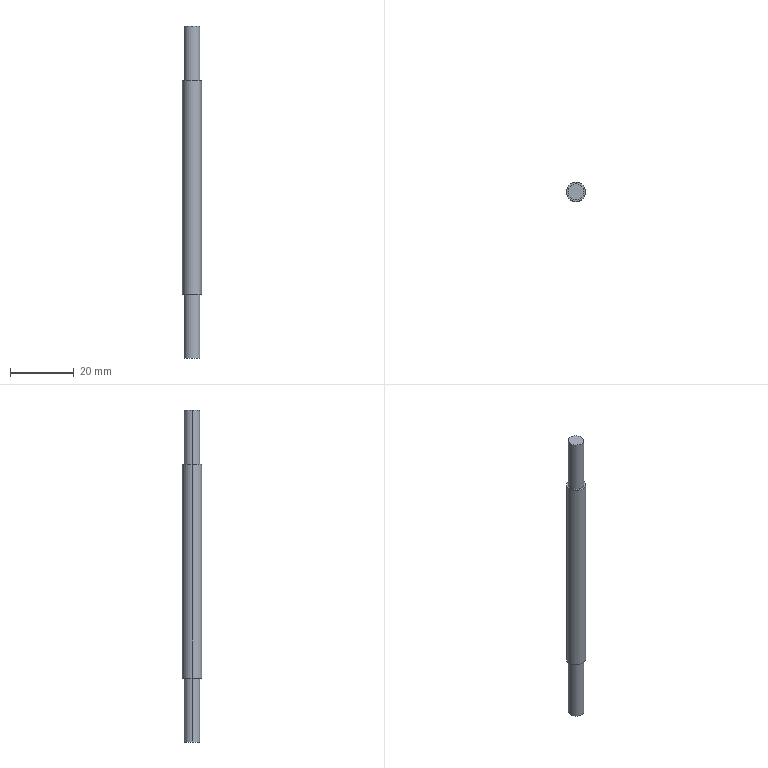Part | SolidWorks | features ICE 2, Extrusion 1 | 1 solid | 10 faces | box 6 x 6 x 104 mm | volume 2621 mm3 | cylinder 6 | plane 4 | commonest cylinder face diameters 5 x4 6 x2
STEP:
#1=CARTESIAN_POINT('',(2.5,0.,104.));
#2=VERTEX_POINT('',#1);
#3=CARTESIAN_POINT('',(-2.5,0.,104.));
#4=VERTEX_POINT('',#3);
#5=CARTESIAN_POINT('',(0.,0.,104.));
#6=DIRECTION('',(0.,0.,1.));
#7=DIRECTION('',(1.,0.,0.));
#8=AXIS2_PLACEMENT_3D('',#5,#6,#7);
#9=CIRCLE('',#8,2.5);
#10=EDGE_CURVE('',#2,#4,#9,.T.);
#11=ORIENTED_EDGE('',*,*,#10,.F.);
#12=CARTESIAN_POINT('',(2.5,0.,87.));
#13=VERTEX_POINT('',#12);
#14=CARTESIAN_POINT('',(2.5,0.,104.));
#15=DIRECTION('',(0.,0.,-1.));
#16=VECTOR('',#15,1000.);
#17=LINE('',#14,#16);
#18=EDGE_CURVE('',#2,#13,#17,.T.);
#19=ORIENTED_EDGE('',*,*,#18,.T.);
#20=CARTESIAN_POINT('',(-2.5,0.,87.));
#21=VERTEX_POINT('',#20);
#22=CARTESIAN_POINT('',(0.,0.,87.));
#23=DIRECTION('',(0.,0.,1.));
#24=DIRECTION('',(1.,0.,0.));
#25=AXIS2_PLACEMENT_3D('',#22,#23,#24);
#26=CIRCLE('',#25,2.5);
#27=EDGE_CURVE('',#13,#21,#26,.T.);
#28=ORIENTED_EDGE('',*,*,#27,.T.);
#29=CARTESIAN_POINT('',(-2.5,0.,104.));
#30=DIRECTION('',(0.,0.,-1.));
#31=VECTOR('',#30,1000.);
#32=LINE('',#29,#31);
#33=EDGE_CURVE('',#4,#21,#32,.T.);
#34=ORIENTED_EDGE('',*,*,#33,.F.);
#35=EDGE_LOOP('',(#11,#19,#28,#34));
#36=FACE_OUTER_BOUND('',#35,.T.);
#37=CARTESIAN_POINT('',(0.,0.,104.));
#38=DIRECTION('',(0.,0.,-1.));
#39=DIRECTION('',(-1.,0.,0.));
#40=AXIS2_PLACEMENT_3D('',#37,#38,#39);
#41=CYLINDRICAL_SURFACE('',#40,2.5);
#42=ADVANCED_FACE('',(#36),#41,.T.);
#43=CARTESIAN_POINT('',(3.,0.,87.));
#44=VERTEX_POINT('',#43);
#45=CARTESIAN_POINT('',(-3.,0.,87.));
#46=VERTEX_POINT('',#45);
#47=CARTESIAN_POINT('',(0.,0.,87.));
#48=DIRECTION('',(0.,0.,1.));
#49=DIRECTION('',(1.,0.,0.));
#50=AXIS2_PLACEMENT_3D('',#47,#48,#49);
#51=CIRCLE('',#50,3.);
#52=EDGE_CURVE('',#44,#46,#51,.T.);
#53=ORIENTED_EDGE('',*,*,#52,.F.);
#54=CARTESIAN_POINT('',(3.,0.,20.));
#55=VERTEX_POINT('',#54);
#56=CARTESIAN_POINT('',(3.,0.,87.));
#57=DIRECTION('',(0.,0.,-1.));
#58=VECTOR('',#57,1000.);
#59=LINE('',#56,#58);
#60=EDGE_CURVE('',#44,#55,#59,.T.);
#61=ORIENTED_EDGE('',*,*,#60,.T.);
#62=CARTESIAN_POINT('',(-3.,0.,20.));
#63=VERTEX_POINT('',#62);
#64=CARTESIAN_POINT('',(0.,0.,20.));
#65=DIRECTION('',(0.,0.,1.));
#66=DIRECTION('',(1.,0.,0.));
#67=AXIS2_PLACEMENT_3D('',#64,#65,#66);
#68=CIRCLE('',#67,3.);
#69=EDGE_CURVE('',#55,#63,#68,.T.);
#70=ORIENTED_EDGE('',*,*,#69,.T.);
#71=CARTESIAN_POINT('',(-3.,0.,87.));
#72=DIRECTION('',(0.,0.,-1.));
#73=VECTOR('',#72,1000.);
#74=LINE('',#71,#73);
#75=EDGE_CURVE('',#46,#63,#74,.T.);
#76=ORIENTED_EDGE('',*,*,#75,.F.);
#77=EDGE_LOOP('',(#53,#61,#70,#76));
#78=FACE_OUTER_BOUND('',#77,.T.);
#79=CARTESIAN_POINT('',(0.,0.,87.));
#80=DIRECTION('',(0.,0.,-1.));
#81=DIRECTION('',(-1.,0.,0.));
#82=AXIS2_PLACEMENT_3D('',#79,#80,#81);
#83=CYLINDRICAL_SURFACE('',#82,3.);
#84=ADVANCED_FACE('',(#78),#83,.T.);
#85=CARTESIAN_POINT('',(2.5,0.,20.));
#86=VERTEX_POINT('',#85);
#87=CARTESIAN_POINT('',(-2.5,0.,20.));
#88=VERTEX_POINT('',#87);
#89=CARTESIAN_POINT('',(0.,0.,20.));
#90=DIRECTION('',(0.,0.,1.));
#91=DIRECTION('',(1.,0.,0.));
#92=AXIS2_PLACEMENT_3D('',#89,#90,#91);
#93=CIRCLE('',#92,2.5);
#94=EDGE_CURVE('',#86,#88,#93,.T.);
#95=ORIENTED_EDGE('',*,*,#94,.F.);
#96=CARTESIAN_POINT('',(2.5,0.,0.));
#97=VERTEX_POINT('',#96);
#98=CARTESIAN_POINT('',(2.5,0.,20.));
#99=DIRECTION('',(0.,0.,-1.));
#100=VECTOR('',#99,1000.);
#101=LINE('',#98,#100);
#102=EDGE_CURVE('',#86,#97,#101,.T.);
#103=ORIENTED_EDGE('',*,*,#102,.T.);
#104=CARTESIAN_POINT('',(-2.5,0.,0.));
#105=VERTEX_POINT('',#104);
#106=CARTESIAN_POINT('',(0.,0.,0.));
#107=DIRECTION('',(0.,0.,1.));
#108=DIRECTION('',(1.,0.,0.));
#109=AXIS2_PLACEMENT_3D('',#106,#107,#108);
#110=CIRCLE('',#109,2.5);
#111=EDGE_CURVE('',#97,#105,#110,.T.);
#112=ORIENTED_EDGE('',*,*,#111,.T.);
#113=CARTESIAN_POINT('',(-2.5,0.,20.));
#114=DIRECTION('',(0.,0.,-1.));
#115=VECTOR('',#114,1000.);
#116=LINE('',#113,#115);
#117=EDGE_CURVE('',#88,#105,#116,.T.);
#118=ORIENTED_EDGE('',*,*,#117,.F.);
#119=EDGE_LOOP('',(#95,#103,#112,#118));
#120=FACE_OUTER_BOUND('',#119,.T.);
#121=CARTESIAN_POINT('',(0.,0.,20.));
#122=DIRECTION('',(0.,0.,-1.));
#123=DIRECTION('',(-1.,0.,0.));
#124=AXIS2_PLACEMENT_3D('',#121,#122,#123);
#125=CYLINDRICAL_SURFACE('',#124,2.5);
#126=ADVANCED_FACE('',(#120),#125,.T.);
#127=ORIENTED_EDGE('',*,*,#102,.F.);
#128=CARTESIAN_POINT('',(0.,0.,20.));
#129=DIRECTION('',(0.,0.,1.));
#130=DIRECTION('',(1.,0.,0.));
#131=AXIS2_PLACEMENT_3D('',#128,#129,#130);
#132=CIRCLE('',#131,2.5);
#133=EDGE_CURVE('',#88,#86,#132,.T.);
#134=ORIENTED_EDGE('',*,*,#133,.F.);
#135=ORIENTED_EDGE('',*,*,#117,.T.);
#136=CARTESIAN_POINT('',(0.,0.,0.));
#137=DIRECTION('',(0.,0.,1.));
#138=DIRECTION('',(1.,0.,0.));
#139=AXIS2_PLACEMENT_3D('',#136,#137,#138);
#140=CIRCLE('',#139,2.5);
#141=EDGE_CURVE('',#105,#97,#140,.T.);
#142=ORIENTED_EDGE('',*,*,#141,.T.);
#143=EDGE_LOOP('',(#127,#134,#135,#142));
#144=FACE_OUTER_BOUND('',#143,.T.);
#145=CARTESIAN_POINT('',(0.,0.,20.));
#146=DIRECTION('',(0.,0.,-1.));
#147=DIRECTION('',(-1.,0.,0.));
#148=AXIS2_PLACEMENT_3D('',#145,#146,#147);
#149=CYLINDRICAL_SURFACE('',#148,2.5);
#150=ADVANCED_FACE('',(#144),#149,.T.);
#151=ORIENTED_EDGE('',*,*,#141,.F.);
#152=ORIENTED_EDGE('',*,*,#111,.F.);
#153=EDGE_LOOP('',(#151,#152));
#154=FACE_OUTER_BOUND('',#153,.T.);
#155=CARTESIAN_POINT('',(0.,0.,0.));
#156=DIRECTION('',(0.,0.,1.));
#157=DIRECTION('',(1.,0.,0.));
#158=AXIS2_PLACEMENT_3D('',#155,#156,#157);
#159=PLANE('',#158);
#160=ADVANCED_FACE('',(#154),#159,.F.);
#161=ORIENTED_EDGE('',*,*,#60,.F.);
#162=CARTESIAN_POINT('',(0.,0.,87.));
#163=DIRECTION('',(0.,0.,1.));
#164=DIRECTION('',(1.,0.,0.));
#165=AXIS2_PLACEMENT_3D('',#162,#163,#164);
#166=CIRCLE('',#165,3.);
#167=EDGE_CURVE('',#46,#44,#166,.T.);
#168=ORIENTED_EDGE('',*,*,#167,.F.);
#169=ORIENTED_EDGE('',*,*,#75,.T.);
#170=CARTESIAN_POINT('',(0.,0.,20.));
#171=DIRECTION('',(0.,0.,1.));
#172=DIRECTION('',(1.,0.,0.));
#173=AXIS2_PLACEMENT_3D('',#170,#171,#172);
#174=CIRCLE('',#173,3.);
#175=EDGE_CURVE('',#63,#55,#174,.T.);
#176=ORIENTED_EDGE('',*,*,#175,.T.);
#177=EDGE_LOOP('',(#161,#168,#169,#176));
#178=FACE_OUTER_BOUND('',#177,.T.);
#179=CARTESIAN_POINT('',(0.,0.,87.));
#180=DIRECTION('',(0.,0.,-1.));
#181=DIRECTION('',(-1.,0.,0.));
#182=AXIS2_PLACEMENT_3D('',#179,#180,#181);
#183=CYLINDRICAL_SURFACE('',#182,3.);
#184=ADVANCED_FACE('',(#178),#183,.T.);
#185=CARTESIAN_POINT('',(0.,0.,87.));
#186=DIRECTION('',(0.,0.,1.));
#187=DIRECTION('',(1.,0.,0.));
#188=AXIS2_PLACEMENT_3D('',#185,#186,#187);
#189=CIRCLE('',#188,2.5);
#190=EDGE_CURVE('',#21,#13,#189,.T.);
#191=ORIENTED_EDGE('',*,*,#190,.F.);
#192=ORIENTED_EDGE('',*,*,#27,.F.);
#193=EDGE_LOOP('',(#191,#192));
#194=FACE_BOUND('',#193,.T.);
#195=ORIENTED_EDGE('',*,*,#167,.T.);
#196=ORIENTED_EDGE('',*,*,#52,.T.);
#197=EDGE_LOOP('',(#195,#196));
#198=FACE_OUTER_BOUND('',#197,.T.);
#199=CARTESIAN_POINT('',(0.,0.,87.));
#200=DIRECTION('',(0.,0.,1.));
#201=DIRECTION('',(1.,0.,0.));
#202=AXIS2_PLACEMENT_3D('',#199,#200,#201);
#203=PLANE('',#202);
#204=ADVANCED_FACE('',(#194,#198),#203,.T.);
#205=ORIENTED_EDGE('',*,*,#133,.T.);
#206=ORIENTED_EDGE('',*,*,#94,.T.);
#207=EDGE_LOOP('',(#205,#206));
#208=FACE_BOUND('',#207,.T.);
#209=ORIENTED_EDGE('',*,*,#175,.F.);
#210=ORIENTED_EDGE('',*,*,#69,.F.);
#211=EDGE_LOOP('',(#209,#210));
#212=FACE_OUTER_BOUND('',#211,.T.);
#213=CARTESIAN_POINT('',(0.,0.,20.));
#214=DIRECTION('',(0.,0.,1.));
#215=DIRECTION('',(1.,0.,0.));
#216=AXIS2_PLACEMENT_3D('',#213,#214,#215);
#217=PLANE('',#216);
#218=ADVANCED_FACE('',(#208,#212),#217,.F.);
#219=ORIENTED_EDGE('',*,*,#18,.F.);
#220=CARTESIAN_POINT('',(0.,0.,104.));
#221=DIRECTION('',(0.,0.,1.));
#222=DIRECTION('',(1.,0.,0.));
#223=AXIS2_PLACEMENT_3D('',#220,#221,#222);
#224=CIRCLE('',#223,2.5);
#225=EDGE_CURVE('',#4,#2,#224,.T.);
#226=ORIENTED_EDGE('',*,*,#225,.F.);
#227=ORIENTED_EDGE('',*,*,#33,.T.);
#228=ORIENTED_EDGE('',*,*,#190,.T.);
#229=EDGE_LOOP('',(#219,#226,#227,#228));
#230=FACE_OUTER_BOUND('',#229,.T.);
#231=CARTESIAN_POINT('',(0.,0.,104.));
#232=DIRECTION('',(0.,0.,-1.));
#233=DIRECTION('',(-1.,0.,0.));
#234=AXIS2_PLACEMENT_3D('',#231,#232,#233);
#235=CYLINDRICAL_SURFACE('',#234,2.5);
#236=ADVANCED_FACE('',(#230),#235,.T.);
#237=ORIENTED_EDGE('',*,*,#225,.T.);
#238=ORIENTED_EDGE('',*,*,#10,.T.);
#239=EDGE_LOOP('',(#237,#238));
#240=FACE_OUTER_BOUND('',#239,.T.);
#241=CARTESIAN_POINT('',(0.,0.,104.));
#242=DIRECTION('',(0.,0.,1.));
#243=DIRECTION('',(1.,0.,0.));
#244=AXIS2_PLACEMENT_3D('',#241,#242,#243);
#245=PLANE('',#244);
#246=ADVANCED_FACE('',(#240),#245,.T.);
#247=CLOSED_SHELL('',(#42,#84,#126,#150,#160,#184,#204,#218,#236,#246));
#248=MANIFOLD_SOLID_BREP('',#247);
#249=CARTESIAN_POINT('',(0.,0.,0.));
#250=DIRECTION('',(0.,0.,1.));
#251=DIRECTION('',(1.,0.,0.));
#252=AXIS2_PLACEMENT_3D('',#249,#250,#251);
#253=(LENGTH_UNIT()NAMED_UNIT(*)SI_UNIT(.MILLI.,.METRE.));
#254=UNCERTAINTY_MEASURE_WITH_UNIT(LENGTH_MEASURE(0.00001),#253,'','');
#255=(NAMED_UNIT(*)PLANE_ANGLE_UNIT()SI_UNIT($,.RADIAN.));
#256=(NAMED_UNIT(*)SI_UNIT($,.STERADIAN.)SOLID_ANGLE_UNIT());
#257=(GEOMETRIC_REPRESENTATION_CONTEXT(3)GLOBAL_UNCERTAINTY_ASSIGNED_CONTEXT((#254))GLOBAL_UNIT_ASSIGNED_CONTEXT((#253,#255,#256))REPRESENTATION_CONTEXT('',''));
#258=ADVANCED_BREP_SHAPE_REPRESENTATION('',(#248,#252),#257);